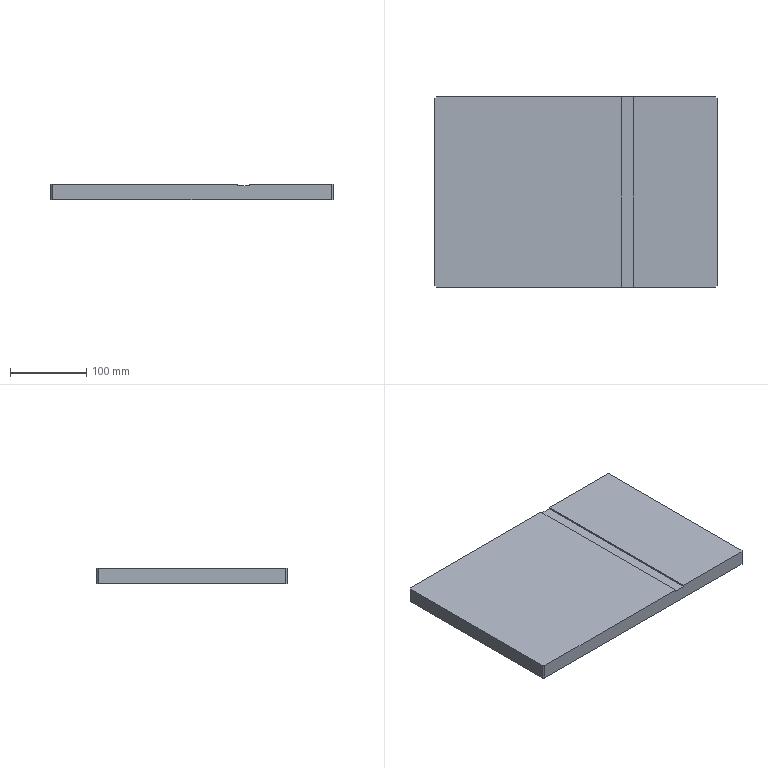Part | STEP file | 001-003-Storage mechanism base plate | 1 solid | 14 faces | box 370 x 250 x 20 mm | volume 1842340 mm3 | plane 14
STEP:
#1=CARTESIAN_POINT('',(0.,0.,0.));
#2=DIRECTION('',(0.,0.,1.));
#3=DIRECTION('',(1.,0.,0.));
#4=AXIS2_PLACEMENT_3D('',#1,#2,#3);
#5=CARTESIAN_POINT('',(183.,125.,20.));
#6=VERTEX_POINT('',#5);
#7=CARTESIAN_POINT('',(75.,125.,20.));
#8=VERTEX_POINT('',#7);
#9=CARTESIAN_POINT('',(-185.,125.,20.));
#10=DIRECTION('',(-1.,0.,0.));
#11=VECTOR('',#10,1.);
#12=LINE('',#9,#11);
#13=CARTESIAN_POINT('',(0.,0.,20.));
#14=DIRECTION('',(0.,0.,-1.));
#15=DIRECTION('',(-1.,0.,0.));
#16=AXIS2_PLACEMENT_3D('',#13,#14,#15);
#17=PLANE('',#16);
#18=CARTESIAN_POINT('',(185.,125.));
#19=DIRECTION('',(1.,0.));
#20=VECTOR('',#19,1.);
#21=LINE('',#18,#20);
#22=(GEOMETRIC_REPRESENTATION_CONTEXT(2)PARAMETRIC_REPRESENTATION_CONTEXT()REPRESENTATION_CONTEXT('',''));
#23=DEFINITIONAL_REPRESENTATION('',(#21),#22);
#24=PCURVE('',#17,#23);
#25=CARTESIAN_POINT('',(-185.,125.,20.));
#26=DIRECTION('',(0.,-1.,0.));
#27=DIRECTION('',(0.,0.,-1.));
#28=AXIS2_PLACEMENT_3D('',#25,#26,#27);
#29=PLANE('',#28);
#30=CARTESIAN_POINT('',(0.,0.));
#31=DIRECTION('',(0.,-1.));
#32=VECTOR('',#31,1.);
#33=LINE('',#30,#32);
#34=(GEOMETRIC_REPRESENTATION_CONTEXT(2)PARAMETRIC_REPRESENTATION_CONTEXT()REPRESENTATION_CONTEXT('',''));
#35=DEFINITIONAL_REPRESENTATION('',(#33),#34);
#36=PCURVE('',#29,#35);
#37=SURFACE_CURVE('',#12,(#24,#36),.PCURVE_S1.);
#38=EDGE_CURVE('',#6,#8,#37,.T.);
#39=ORIENTED_EDGE('',*,*,#38,.T.);
#40=CARTESIAN_POINT('',(75.,-125.,20.));
#41=VERTEX_POINT('',#40);
#42=CARTESIAN_POINT('',(75.,125.,20.));
#43=DIRECTION('',(0.,1.,0.));
#44=VECTOR('',#43,1.);
#45=LINE('',#42,#44);
#46=CARTESIAN_POINT('',(-75.,125.));
#47=DIRECTION('',(0.,1.));
#48=VECTOR('',#47,1.);
#49=LINE('',#46,#48);
#50=(GEOMETRIC_REPRESENTATION_CONTEXT(2)PARAMETRIC_REPRESENTATION_CONTEXT()REPRESENTATION_CONTEXT('',''));
#51=DEFINITIONAL_REPRESENTATION('',(#49),#50);
#52=PCURVE('',#17,#51);
#53=CARTESIAN_POINT('',(75.,125.,18.));
#54=DIRECTION('',(1.,0.,0.));
#55=DIRECTION('',(0.,1.,0.));
#56=AXIS2_PLACEMENT_3D('',#53,#54,#55);
#57=PLANE('',#56);
#58=CARTESIAN_POINT('',(0.,2.));
#59=DIRECTION('',(1.,0.));
#60=VECTOR('',#59,1.);
#61=LINE('',#58,#60);
#62=(GEOMETRIC_REPRESENTATION_CONTEXT(2)PARAMETRIC_REPRESENTATION_CONTEXT()REPRESENTATION_CONTEXT('',''));
#63=DEFINITIONAL_REPRESENTATION('',(#61),#62);
#64=PCURVE('',#57,#63);
#65=SURFACE_CURVE('',#45,(#52,#64),.PCURVE_S1.);
#66=EDGE_CURVE('',#41,#8,#65,.T.);
#67=ORIENTED_EDGE('',*,*,#66,.F.);
#68=CARTESIAN_POINT('',(183.,-125.,20.));
#69=VERTEX_POINT('',#68);
#70=CARTESIAN_POINT('',(-185.,-125.,20.));
#71=DIRECTION('',(1.,0.,0.));
#72=VECTOR('',#71,1.);
#73=LINE('',#70,#72);
#74=CARTESIAN_POINT('',(185.,-125.));
#75=DIRECTION('',(-1.,0.));
#76=VECTOR('',#75,1.);
#77=LINE('',#74,#76);
#78=(GEOMETRIC_REPRESENTATION_CONTEXT(2)PARAMETRIC_REPRESENTATION_CONTEXT()REPRESENTATION_CONTEXT('',''));
#79=DEFINITIONAL_REPRESENTATION('',(#77),#78);
#80=PCURVE('',#17,#79);
#81=CARTESIAN_POINT('',(-185.,-125.,20.));
#82=DIRECTION('',(0.,1.,0.));
#83=DIRECTION('',(0.,0.,1.));
#84=AXIS2_PLACEMENT_3D('',#81,#82,#83);
#85=PLANE('',#84);
#86=CARTESIAN_POINT('',(0.,0.));
#87=DIRECTION('',(0.,1.));
#88=VECTOR('',#87,1.);
#89=LINE('',#86,#88);
#90=(GEOMETRIC_REPRESENTATION_CONTEXT(2)PARAMETRIC_REPRESENTATION_CONTEXT()REPRESENTATION_CONTEXT('',''));
#91=DEFINITIONAL_REPRESENTATION('',(#89),#90);
#92=PCURVE('',#85,#91);
#93=SURFACE_CURVE('',#73,(#80,#92),.PCURVE_S1.);
#94=EDGE_CURVE('',#41,#69,#93,.T.);
#95=ORIENTED_EDGE('',*,*,#94,.T.);
#96=CARTESIAN_POINT('',(185.,-123.,20.));
#97=VERTEX_POINT('',#96);
#98=CARTESIAN_POINT('',(185.,-123.,20.));
#99=DIRECTION('',(0.7071,0.7071,0.));
#100=VECTOR('',#99,1.);
#101=LINE('',#98,#100);
#102=CARTESIAN_POINT('',(-185.,-123.));
#103=DIRECTION('',(-0.7071,0.7071));
#104=VECTOR('',#103,1.);
#105=LINE('',#102,#104);
#106=(GEOMETRIC_REPRESENTATION_CONTEXT(2)PARAMETRIC_REPRESENTATION_CONTEXT()REPRESENTATION_CONTEXT('',''));
#107=DEFINITIONAL_REPRESENTATION('',(#105),#106);
#108=PCURVE('',#17,#107);
#109=CARTESIAN_POINT('',(185.,-123.,20.));
#110=DIRECTION('',(-0.7071,0.7071,0.));
#111=DIRECTION('',(0.,0.,-1.));
#112=AXIS2_PLACEMENT_3D('',#109,#110,#111);
#113=PLANE('',#112);
#114=CARTESIAN_POINT('',(0.,0.));
#115=DIRECTION('',(0.,-1.));
#116=VECTOR('',#115,1.);
#117=LINE('',#114,#116);
#118=(GEOMETRIC_REPRESENTATION_CONTEXT(2)PARAMETRIC_REPRESENTATION_CONTEXT()REPRESENTATION_CONTEXT('',''));
#119=DEFINITIONAL_REPRESENTATION('',(#117),#118);
#120=PCURVE('',#113,#119);
#121=SURFACE_CURVE('',#101,(#108,#120),.PCURVE_S1.);
#122=EDGE_CURVE('',#69,#97,#121,.T.);
#123=ORIENTED_EDGE('',*,*,#122,.T.);
#124=CARTESIAN_POINT('',(185.,123.,20.));
#125=VERTEX_POINT('',#124);
#126=CARTESIAN_POINT('',(185.,-125.,20.));
#127=DIRECTION('',(0.,1.,0.));
#128=VECTOR('',#127,1.);
#129=LINE('',#126,#128);
#130=CARTESIAN_POINT('',(-185.,-125.));
#131=DIRECTION('',(0.,1.));
#132=VECTOR('',#131,1.);
#133=LINE('',#130,#132);
#134=(GEOMETRIC_REPRESENTATION_CONTEXT(2)PARAMETRIC_REPRESENTATION_CONTEXT()REPRESENTATION_CONTEXT('',''));
#135=DEFINITIONAL_REPRESENTATION('',(#133),#134);
#136=PCURVE('',#17,#135);
#137=CARTESIAN_POINT('',(185.,-125.,20.));
#138=DIRECTION('',(-1.,0.,0.));
#139=DIRECTION('',(0.,0.,1.));
#140=AXIS2_PLACEMENT_3D('',#137,#138,#139);
#141=PLANE('',#140);
#142=CARTESIAN_POINT('',(0.,0.));
#143=DIRECTION('',(0.,1.));
#144=VECTOR('',#143,1.);
#145=LINE('',#142,#144);
#146=(GEOMETRIC_REPRESENTATION_CONTEXT(2)PARAMETRIC_REPRESENTATION_CONTEXT()REPRESENTATION_CONTEXT('',''));
#147=DEFINITIONAL_REPRESENTATION('',(#145),#146);
#148=PCURVE('',#141,#147);
#149=SURFACE_CURVE('',#129,(#136,#148),.PCURVE_S1.);
#150=EDGE_CURVE('',#97,#125,#149,.T.);
#151=ORIENTED_EDGE('',*,*,#150,.T.);
#152=CARTESIAN_POINT('',(183.,125.,20.));
#153=DIRECTION('',(-0.7071,0.7071,0.));
#154=VECTOR('',#153,1.);
#155=LINE('',#152,#154);
#156=CARTESIAN_POINT('',(-183.,125.));
#157=DIRECTION('',(0.7071,0.7071));
#158=VECTOR('',#157,1.);
#159=LINE('',#156,#158);
#160=(GEOMETRIC_REPRESENTATION_CONTEXT(2)PARAMETRIC_REPRESENTATION_CONTEXT()REPRESENTATION_CONTEXT('',''));
#161=DEFINITIONAL_REPRESENTATION('',(#159),#160);
#162=PCURVE('',#17,#161);
#163=CARTESIAN_POINT('',(183.,125.,20.));
#164=DIRECTION('',(-0.7071,-0.7071,0.));
#165=DIRECTION('',(0.,0.,-1.));
#166=AXIS2_PLACEMENT_3D('',#163,#164,#165);
#167=PLANE('',#166);
#168=CARTESIAN_POINT('',(0.,0.));
#169=DIRECTION('',(0.,-1.));
#170=VECTOR('',#169,1.);
#171=LINE('',#168,#170);
#172=(GEOMETRIC_REPRESENTATION_CONTEXT(2)PARAMETRIC_REPRESENTATION_CONTEXT()REPRESENTATION_CONTEXT('',''));
#173=DEFINITIONAL_REPRESENTATION('',(#171),#172);
#174=PCURVE('',#167,#173);
#175=SURFACE_CURVE('',#155,(#162,#174),.PCURVE_S1.);
#176=EDGE_CURVE('',#125,#6,#175,.T.);
#177=ORIENTED_EDGE('',*,*,#176,.T.);
#178=EDGE_LOOP('',(#39,#67,#95,#123,#151,#177));
#179=FACE_BOUND('',#178,.T.);
#180=ADVANCED_FACE('',(#179),#17,.F.);
#181=ORIENTED_EDGE('',*,*,#150,.F.);
#182=CARTESIAN_POINT('',(185.,-123.,0.));
#183=VERTEX_POINT('',#182);
#184=CARTESIAN_POINT('',(185.,-123.,20.));
#185=DIRECTION('',(0.,0.,-1.));
#186=VECTOR('',#185,1.);
#187=LINE('',#184,#186);
#188=CARTESIAN_POINT('',(0.,2.));
#189=DIRECTION('',(-1.,0.));
#190=VECTOR('',#189,1.);
#191=LINE('',#188,#190);
#192=(GEOMETRIC_REPRESENTATION_CONTEXT(2)PARAMETRIC_REPRESENTATION_CONTEXT()REPRESENTATION_CONTEXT('',''));
#193=DEFINITIONAL_REPRESENTATION('',(#191),#192);
#194=PCURVE('',#141,#193);
#195=CARTESIAN_POINT('',(0.,0.));
#196=DIRECTION('',(1.,0.));
#197=VECTOR('',#196,1.);
#198=LINE('',#195,#197);
#199=(GEOMETRIC_REPRESENTATION_CONTEXT(2)PARAMETRIC_REPRESENTATION_CONTEXT()REPRESENTATION_CONTEXT('',''));
#200=DEFINITIONAL_REPRESENTATION('',(#198),#199);
#201=PCURVE('',#113,#200);
#202=SURFACE_CURVE('',#187,(#194,#201),.PCURVE_S1.);
#203=EDGE_CURVE('',#97,#183,#202,.T.);
#204=ORIENTED_EDGE('',*,*,#203,.T.);
#205=CARTESIAN_POINT('',(185.,123.,0.));
#206=VERTEX_POINT('',#205);
#207=CARTESIAN_POINT('',(185.,-125.,0.));
#208=DIRECTION('',(0.,1.,0.));
#209=VECTOR('',#208,1.);
#210=LINE('',#207,#209);
#211=CARTESIAN_POINT('',(-20.,0.));
#212=DIRECTION('',(0.,1.));
#213=VECTOR('',#212,1.);
#214=LINE('',#211,#213);
#215=(GEOMETRIC_REPRESENTATION_CONTEXT(2)PARAMETRIC_REPRESENTATION_CONTEXT()REPRESENTATION_CONTEXT('',''));
#216=DEFINITIONAL_REPRESENTATION('',(#214),#215);
#217=PCURVE('',#141,#216);
#218=CARTESIAN_POINT('',(0.,0.,0.));
#219=DIRECTION('',(0.,0.,-1.));
#220=DIRECTION('',(-1.,0.,0.));
#221=AXIS2_PLACEMENT_3D('',#218,#219,#220);
#222=PLANE('',#221);
#223=CARTESIAN_POINT('',(-185.,-125.));
#224=DIRECTION('',(0.,1.));
#225=VECTOR('',#224,1.);
#226=LINE('',#223,#225);
#227=(GEOMETRIC_REPRESENTATION_CONTEXT(2)PARAMETRIC_REPRESENTATION_CONTEXT()REPRESENTATION_CONTEXT('',''));
#228=DEFINITIONAL_REPRESENTATION('',(#226),#227);
#229=PCURVE('',#222,#228);
#230=SURFACE_CURVE('',#210,(#217,#229),.PCURVE_S1.);
#231=EDGE_CURVE('',#183,#206,#230,.T.);
#232=ORIENTED_EDGE('',*,*,#231,.T.);
#233=CARTESIAN_POINT('',(185.,123.,20.));
#234=DIRECTION('',(0.,0.,1.));
#235=VECTOR('',#234,1.);
#236=LINE('',#233,#235);
#237=CARTESIAN_POINT('',(0.,248.));
#238=DIRECTION('',(1.,0.));
#239=VECTOR('',#238,1.);
#240=LINE('',#237,#239);
#241=(GEOMETRIC_REPRESENTATION_CONTEXT(2)PARAMETRIC_REPRESENTATION_CONTEXT()REPRESENTATION_CONTEXT('',''));
#242=DEFINITIONAL_REPRESENTATION('',(#240),#241);
#243=PCURVE('',#141,#242);
#244=CARTESIAN_POINT('',(0.,2.828));
#245=DIRECTION('',(-1.,0.));
#246=VECTOR('',#245,1.);
#247=LINE('',#244,#246);
#248=(GEOMETRIC_REPRESENTATION_CONTEXT(2)PARAMETRIC_REPRESENTATION_CONTEXT()REPRESENTATION_CONTEXT('',''));
#249=DEFINITIONAL_REPRESENTATION('',(#247),#248);
#250=PCURVE('',#167,#249);
#251=SURFACE_CURVE('',#236,(#243,#250),.PCURVE_S1.);
#252=EDGE_CURVE('',#206,#125,#251,.T.);
#253=ORIENTED_EDGE('',*,*,#252,.T.);
#254=EDGE_LOOP('',(#181,#204,#232,#253));
#255=FACE_BOUND('',#254,.T.);
#256=ADVANCED_FACE('',(#255),#141,.F.);
#257=CARTESIAN_POINT('',(75.,125.,18.));
#258=VERTEX_POINT('',#257);
#259=CARTESIAN_POINT('',(60.,125.,18.));
#260=VERTEX_POINT('',#259);
#261=CARTESIAN_POINT('',(75.,125.,18.));
#262=DIRECTION('',(-1.,0.,0.));
#263=VECTOR('',#262,1.);
#264=LINE('',#261,#263);
#265=CARTESIAN_POINT('',(2.,260.));
#266=DIRECTION('',(0.,-1.));
#267=VECTOR('',#266,1.);
#268=LINE('',#265,#267);
#269=(GEOMETRIC_REPRESENTATION_CONTEXT(2)PARAMETRIC_REPRESENTATION_CONTEXT()REPRESENTATION_CONTEXT('',''));
#270=DEFINITIONAL_REPRESENTATION('',(#268),#269);
#271=PCURVE('',#29,#270);
#272=CARTESIAN_POINT('',(0.,0.,18.));
#273=DIRECTION('',(0.,0.,-1.));
#274=DIRECTION('',(-1.,0.,0.));
#275=AXIS2_PLACEMENT_3D('',#272,#273,#274);
#276=PLANE('',#275);
#277=CARTESIAN_POINT('',(-75.,125.));
#278=DIRECTION('',(1.,0.));
#279=VECTOR('',#278,1.);
#280=LINE('',#277,#279);
#281=(GEOMETRIC_REPRESENTATION_CONTEXT(2)PARAMETRIC_REPRESENTATION_CONTEXT()REPRESENTATION_CONTEXT('',''));
#282=DEFINITIONAL_REPRESENTATION('',(#280),#281);
#283=PCURVE('',#276,#282);
#284=SURFACE_CURVE('',#264,(#271,#283),.PCURVE_S1.);
#285=EDGE_CURVE('',#258,#260,#284,.T.);
#286=ORIENTED_EDGE('',*,*,#285,.F.);
#287=CARTESIAN_POINT('',(75.,125.,18.));
#288=DIRECTION('',(0.,0.,1.));
#289=VECTOR('',#288,1.);
#290=LINE('',#287,#289);
#291=CARTESIAN_POINT('',(2.,260.));
#292=DIRECTION('',(-1.,0.));
#293=VECTOR('',#292,1.);
#294=LINE('',#291,#293);
#295=(GEOMETRIC_REPRESENTATION_CONTEXT(2)PARAMETRIC_REPRESENTATION_CONTEXT()REPRESENTATION_CONTEXT('',''));
#296=DEFINITIONAL_REPRESENTATION('',(#294),#295);
#297=PCURVE('',#29,#296);
#298=CARTESIAN_POINT('',(0.,0.));
#299=DIRECTION('',(0.,1.));
#300=VECTOR('',#299,1.);
#301=LINE('',#298,#300);
#302=(GEOMETRIC_REPRESENTATION_CONTEXT(2)PARAMETRIC_REPRESENTATION_CONTEXT()REPRESENTATION_CONTEXT('',''));
#303=DEFINITIONAL_REPRESENTATION('',(#301),#302);
#304=PCURVE('',#57,#303);
#305=SURFACE_CURVE('',#290,(#297,#304),.PCURVE_S1.);
#306=EDGE_CURVE('',#258,#8,#305,.T.);
#307=ORIENTED_EDGE('',*,*,#306,.T.);
#308=ORIENTED_EDGE('',*,*,#38,.F.);
#309=CARTESIAN_POINT('',(183.,125.,0.));
#310=VERTEX_POINT('',#309);
#311=CARTESIAN_POINT('',(183.,125.,20.));
#312=DIRECTION('',(0.,0.,-1.));
#313=VECTOR('',#312,1.);
#314=LINE('',#311,#313);
#315=CARTESIAN_POINT('',(0.,368.));
#316=DIRECTION('',(1.,0.));
#317=VECTOR('',#316,1.);
#318=LINE('',#315,#317);
#319=(GEOMETRIC_REPRESENTATION_CONTEXT(2)PARAMETRIC_REPRESENTATION_CONTEXT()REPRESENTATION_CONTEXT('',''));
#320=DEFINITIONAL_REPRESENTATION('',(#318),#319);
#321=PCURVE('',#29,#320);
#322=CARTESIAN_POINT('',(0.,0.));
#323=DIRECTION('',(1.,0.));
#324=VECTOR('',#323,1.);
#325=LINE('',#322,#324);
#326=(GEOMETRIC_REPRESENTATION_CONTEXT(2)PARAMETRIC_REPRESENTATION_CONTEXT()REPRESENTATION_CONTEXT('',''));
#327=DEFINITIONAL_REPRESENTATION('',(#325),#326);
#328=PCURVE('',#167,#327);
#329=SURFACE_CURVE('',#314,(#321,#328),.PCURVE_S1.);
#330=EDGE_CURVE('',#6,#310,#329,.T.);
#331=ORIENTED_EDGE('',*,*,#330,.T.);
#332=CARTESIAN_POINT('',(-183.,125.,0.));
#333=VERTEX_POINT('',#332);
#334=CARTESIAN_POINT('',(-185.,125.,0.));
#335=DIRECTION('',(-1.,0.,0.));
#336=VECTOR('',#335,1.);
#337=LINE('',#334,#336);
#338=CARTESIAN_POINT('',(20.,0.));
#339=DIRECTION('',(0.,-1.));
#340=VECTOR('',#339,1.);
#341=LINE('',#338,#340);
#342=(GEOMETRIC_REPRESENTATION_CONTEXT(2)PARAMETRIC_REPRESENTATION_CONTEXT()REPRESENTATION_CONTEXT('',''));
#343=DEFINITIONAL_REPRESENTATION('',(#341),#342);
#344=PCURVE('',#29,#343);
#345=CARTESIAN_POINT('',(185.,125.));
#346=DIRECTION('',(1.,0.));
#347=VECTOR('',#346,1.);
#348=LINE('',#345,#347);
#349=(GEOMETRIC_REPRESENTATION_CONTEXT(2)PARAMETRIC_REPRESENTATION_CONTEXT()REPRESENTATION_CONTEXT('',''));
#350=DEFINITIONAL_REPRESENTATION('',(#348),#349);
#351=PCURVE('',#222,#350);
#352=SURFACE_CURVE('',#337,(#344,#351),.PCURVE_S1.);
#353=EDGE_CURVE('',#310,#333,#352,.T.);
#354=ORIENTED_EDGE('',*,*,#353,.T.);
#355=CARTESIAN_POINT('',(-183.,125.,20.));
#356=VERTEX_POINT('',#355);
#357=CARTESIAN_POINT('',(-183.,125.,20.));
#358=DIRECTION('',(0.,0.,1.));
#359=VECTOR('',#358,1.);
#360=LINE('',#357,#359);
#361=CARTESIAN_POINT('',(0.,2.));
#362=DIRECTION('',(-1.,0.));
#363=VECTOR('',#362,1.);
#364=LINE('',#361,#363);
#365=(GEOMETRIC_REPRESENTATION_CONTEXT(2)PARAMETRIC_REPRESENTATION_CONTEXT()REPRESENTATION_CONTEXT('',''));
#366=DEFINITIONAL_REPRESENTATION('',(#364),#365);
#367=PCURVE('',#29,#366);
#368=CARTESIAN_POINT('',(-185.,123.,20.));
#369=DIRECTION('',(0.7071,-0.7071,0.));
#370=DIRECTION('',(0.,0.,-1.));
#371=AXIS2_PLACEMENT_3D('',#368,#369,#370);
#372=PLANE('',#371);
#373=CARTESIAN_POINT('',(0.,2.828));
#374=DIRECTION('',(-1.,0.));
#375=VECTOR('',#374,1.);
#376=LINE('',#373,#375);
#377=(GEOMETRIC_REPRESENTATION_CONTEXT(2)PARAMETRIC_REPRESENTATION_CONTEXT()REPRESENTATION_CONTEXT('',''));
#378=DEFINITIONAL_REPRESENTATION('',(#376),#377);
#379=PCURVE('',#372,#378);
#380=SURFACE_CURVE('',#360,(#367,#379),.PCURVE_S1.);
#381=EDGE_CURVE('',#333,#356,#380,.T.);
#382=ORIENTED_EDGE('',*,*,#381,.T.);
#383=CARTESIAN_POINT('',(60.,125.,20.));
#384=VERTEX_POINT('',#383);
#385=CARTESIAN_POINT('',(-185.,125.,20.));
#386=DIRECTION('',(-1.,0.,0.));
#387=VECTOR('',#386,1.);
#388=LINE('',#385,#387);
#389=CARTESIAN_POINT('',(0.,0.));
#390=DIRECTION('',(0.,-1.));
#391=VECTOR('',#390,1.);
#392=LINE('',#389,#391);
#393=(GEOMETRIC_REPRESENTATION_CONTEXT(2)PARAMETRIC_REPRESENTATION_CONTEXT()REPRESENTATION_CONTEXT('',''));
#394=DEFINITIONAL_REPRESENTATION('',(#392),#393);
#395=PCURVE('',#29,#394);
#396=CARTESIAN_POINT('',(0.,0.,20.));
#397=DIRECTION('',(0.,0.,-1.));
#398=DIRECTION('',(-1.,0.,0.));
#399=AXIS2_PLACEMENT_3D('',#396,#397,#398);
#400=PLANE('',#399);
#401=CARTESIAN_POINT('',(185.,125.));
#402=DIRECTION('',(1.,0.));
#403=VECTOR('',#402,1.);
#404=LINE('',#401,#403);
#405=(GEOMETRIC_REPRESENTATION_CONTEXT(2)PARAMETRIC_REPRESENTATION_CONTEXT()REPRESENTATION_CONTEXT('',''));
#406=DEFINITIONAL_REPRESENTATION('',(#404),#405);
#407=PCURVE('',#400,#406);
#408=SURFACE_CURVE('',#388,(#395,#407),.PCURVE_S1.);
#409=EDGE_CURVE('',#384,#356,#408,.T.);
#410=ORIENTED_EDGE('',*,*,#409,.F.);
#411=CARTESIAN_POINT('',(60.,125.,18.));
#412=DIRECTION('',(0.,0.,1.));
#413=VECTOR('',#412,1.);
#414=LINE('',#411,#413);
#415=CARTESIAN_POINT('',(2.,245.));
#416=DIRECTION('',(-1.,0.));
#417=VECTOR('',#416,1.);
#418=LINE('',#415,#417);
#419=(GEOMETRIC_REPRESENTATION_CONTEXT(2)PARAMETRIC_REPRESENTATION_CONTEXT()REPRESENTATION_CONTEXT('',''));
#420=DEFINITIONAL_REPRESENTATION('',(#418),#419);
#421=PCURVE('',#29,#420);
#422=CARTESIAN_POINT('',(60.,125.,18.));
#423=DIRECTION('',(-1.,0.,0.));
#424=DIRECTION('',(0.,-1.,0.));
#425=AXIS2_PLACEMENT_3D('',#422,#423,#424);
#426=PLANE('',#425);
#427=CARTESIAN_POINT('',(0.,0.));
#428=DIRECTION('',(0.,1.));
#429=VECTOR('',#428,1.);
#430=LINE('',#427,#429);
#431=(GEOMETRIC_REPRESENTATION_CONTEXT(2)PARAMETRIC_REPRESENTATION_CONTEXT()REPRESENTATION_CONTEXT('',''));
#432=DEFINITIONAL_REPRESENTATION('',(#430),#431);
#433=PCURVE('',#426,#432);
#434=SURFACE_CURVE('',#414,(#421,#433),.PCURVE_S1.);
#435=EDGE_CURVE('',#260,#384,#434,.T.);
#436=ORIENTED_EDGE('',*,*,#435,.F.);
#437=EDGE_LOOP('',(#286,#307,#308,#331,#354,#382,#410,#436));
#438=FACE_BOUND('',#437,.T.);
#439=ADVANCED_FACE('',(#438),#29,.F.);
#440=CARTESIAN_POINT('',(-185.,123.,0.));
#441=VERTEX_POINT('',#440);
#442=CARTESIAN_POINT('',(-185.,-123.,0.));
#443=VERTEX_POINT('',#442);
#444=CARTESIAN_POINT('',(-185.,-125.,0.));
#445=DIRECTION('',(0.,-1.,0.));
#446=VECTOR('',#445,1.);
#447=LINE('',#444,#446);
#448=CARTESIAN_POINT('',(-185.,-125.,20.));
#449=DIRECTION('',(1.,0.,0.));
#450=DIRECTION('',(0.,0.,-1.));
#451=AXIS2_PLACEMENT_3D('',#448,#449,#450);
#452=PLANE('',#451);
#453=CARTESIAN_POINT('',(20.,0.));
#454=DIRECTION('',(0.,-1.));
#455=VECTOR('',#454,1.);
#456=LINE('',#453,#455);
#457=(GEOMETRIC_REPRESENTATION_CONTEXT(2)PARAMETRIC_REPRESENTATION_CONTEXT()REPRESENTATION_CONTEXT('',''));
#458=DEFINITIONAL_REPRESENTATION('',(#456),#457);
#459=PCURVE('',#452,#458);
#460=CARTESIAN_POINT('',(185.,-125.));
#461=DIRECTION('',(0.,-1.));
#462=VECTOR('',#461,1.);
#463=LINE('',#460,#462);
#464=(GEOMETRIC_REPRESENTATION_CONTEXT(2)PARAMETRIC_REPRESENTATION_CONTEXT()REPRESENTATION_CONTEXT('',''));
#465=DEFINITIONAL_REPRESENTATION('',(#463),#464);
#466=PCURVE('',#222,#465);
#467=SURFACE_CURVE('',#447,(#459,#466),.PCURVE_S1.);
#468=EDGE_CURVE('',#441,#443,#467,.T.);
#469=ORIENTED_EDGE('',*,*,#468,.T.);
#470=CARTESIAN_POINT('',(-185.,-123.,20.));
#471=VERTEX_POINT('',#470);
#472=CARTESIAN_POINT('',(-185.,-123.,20.));
#473=DIRECTION('',(0.,0.,1.));
#474=VECTOR('',#473,1.);
#475=LINE('',#472,#474);
#476=CARTESIAN_POINT('',(0.,2.));
#477=DIRECTION('',(-1.,0.));
#478=VECTOR('',#477,1.);
#479=LINE('',#476,#478);
#480=(GEOMETRIC_REPRESENTATION_CONTEXT(2)PARAMETRIC_REPRESENTATION_CONTEXT()REPRESENTATION_CONTEXT('',''));
#481=DEFINITIONAL_REPRESENTATION('',(#479),#480);
#482=PCURVE('',#452,#481);
#483=CARTESIAN_POINT('',(-183.,-125.,20.));
#484=DIRECTION('',(0.7071,0.7071,0.));
#485=DIRECTION('',(0.,0.,-1.));
#486=AXIS2_PLACEMENT_3D('',#483,#484,#485);
#487=PLANE('',#486);
#488=CARTESIAN_POINT('',(0.,2.828));
#489=DIRECTION('',(-1.,0.));
#490=VECTOR('',#489,1.);
#491=LINE('',#488,#490);
#492=(GEOMETRIC_REPRESENTATION_CONTEXT(2)PARAMETRIC_REPRESENTATION_CONTEXT()REPRESENTATION_CONTEXT('',''));
#493=DEFINITIONAL_REPRESENTATION('',(#491),#492);
#494=PCURVE('',#487,#493);
#495=SURFACE_CURVE('',#475,(#482,#494),.PCURVE_S1.);
#496=EDGE_CURVE('',#443,#471,#495,.T.);
#497=ORIENTED_EDGE('',*,*,#496,.T.);
#498=CARTESIAN_POINT('',(-185.,123.,20.));
#499=VERTEX_POINT('',#498);
#500=CARTESIAN_POINT('',(-185.,-125.,20.));
#501=DIRECTION('',(0.,-1.,0.));
#502=VECTOR('',#501,1.);
#503=LINE('',#500,#502);
#504=CARTESIAN_POINT('',(0.,0.));
#505=DIRECTION('',(0.,-1.));
#506=VECTOR('',#505,1.);
#507=LINE('',#504,#506);
#508=(GEOMETRIC_REPRESENTATION_CONTEXT(2)PARAMETRIC_REPRESENTATION_CONTEXT()REPRESENTATION_CONTEXT('',''));
#509=DEFINITIONAL_REPRESENTATION('',(#507),#508);
#510=PCURVE('',#452,#509);
#511=CARTESIAN_POINT('',(185.,-125.));
#512=DIRECTION('',(0.,-1.));
#513=VECTOR('',#512,1.);
#514=LINE('',#511,#513);
#515=(GEOMETRIC_REPRESENTATION_CONTEXT(2)PARAMETRIC_REPRESENTATION_CONTEXT()REPRESENTATION_CONTEXT('',''));
#516=DEFINITIONAL_REPRESENTATION('',(#514),#515);
#517=PCURVE('',#400,#516);
#518=SURFACE_CURVE('',#503,(#510,#517),.PCURVE_S1.);
#519=EDGE_CURVE('',#499,#471,#518,.T.);
#520=ORIENTED_EDGE('',*,*,#519,.F.);
#521=CARTESIAN_POINT('',(-185.,123.,20.));
#522=DIRECTION('',(0.,0.,-1.));
#523=VECTOR('',#522,1.);
#524=LINE('',#521,#523);
#525=CARTESIAN_POINT('',(0.,248.));
#526=DIRECTION('',(1.,0.));
#527=VECTOR('',#526,1.);
#528=LINE('',#525,#527);
#529=(GEOMETRIC_REPRESENTATION_CONTEXT(2)PARAMETRIC_REPRESENTATION_CONTEXT()REPRESENTATION_CONTEXT('',''));
#530=DEFINITIONAL_REPRESENTATION('',(#528),#529);
#531=PCURVE('',#452,#530);
#532=CARTESIAN_POINT('',(0.,0.));
#533=DIRECTION('',(1.,0.));
#534=VECTOR('',#533,1.);
#535=LINE('',#532,#534);
#536=(GEOMETRIC_REPRESENTATION_CONTEXT(2)PARAMETRIC_REPRESENTATION_CONTEXT()REPRESENTATION_CONTEXT('',''));
#537=DEFINITIONAL_REPRESENTATION('',(#535),#536);
#538=PCURVE('',#372,#537);
#539=SURFACE_CURVE('',#524,(#531,#538),.PCURVE_S1.);
#540=EDGE_CURVE('',#499,#441,#539,.T.);
#541=ORIENTED_EDGE('',*,*,#540,.T.);
#542=EDGE_LOOP('',(#469,#497,#520,#541));
#543=FACE_BOUND('',#542,.T.);
#544=ADVANCED_FACE('',(#543),#452,.F.);
#545=ORIENTED_EDGE('',*,*,#94,.F.);
#546=CARTESIAN_POINT('',(75.,-125.,18.));
#547=VERTEX_POINT('',#546);
#548=CARTESIAN_POINT('',(75.,-125.,18.));
#549=DIRECTION('',(0.,0.,1.));
#550=VECTOR('',#549,1.);
#551=LINE('',#548,#550);
#552=CARTESIAN_POINT('',(-2.,260.));
#553=DIRECTION('',(1.,0.));
#554=VECTOR('',#553,1.);
#555=LINE('',#552,#554);
#556=(GEOMETRIC_REPRESENTATION_CONTEXT(2)PARAMETRIC_REPRESENTATION_CONTEXT()REPRESENTATION_CONTEXT('',''));
#557=DEFINITIONAL_REPRESENTATION('',(#555),#556);
#558=PCURVE('',#85,#557);
#559=CARTESIAN_POINT('',(-250.,0.));
#560=DIRECTION('',(0.,1.));
#561=VECTOR('',#560,1.);
#562=LINE('',#559,#561);
#563=(GEOMETRIC_REPRESENTATION_CONTEXT(2)PARAMETRIC_REPRESENTATION_CONTEXT()REPRESENTATION_CONTEXT('',''));
#564=DEFINITIONAL_REPRESENTATION('',(#562),#563);
#565=PCURVE('',#57,#564);
#566=SURFACE_CURVE('',#551,(#558,#565),.PCURVE_S1.);
#567=EDGE_CURVE('',#547,#41,#566,.T.);
#568=ORIENTED_EDGE('',*,*,#567,.F.);
#569=CARTESIAN_POINT('',(60.,-125.,18.));
#570=VERTEX_POINT('',#569);
#571=CARTESIAN_POINT('',(75.,-125.,18.));
#572=DIRECTION('',(1.,0.,0.));
#573=VECTOR('',#572,1.);
#574=LINE('',#571,#573);
#575=CARTESIAN_POINT('',(-2.,260.));
#576=DIRECTION('',(0.,1.));
#577=VECTOR('',#576,1.);
#578=LINE('',#575,#577);
#579=(GEOMETRIC_REPRESENTATION_CONTEXT(2)PARAMETRIC_REPRESENTATION_CONTEXT()REPRESENTATION_CONTEXT('',''));
#580=DEFINITIONAL_REPRESENTATION('',(#578),#579);
#581=PCURVE('',#85,#580);
#582=CARTESIAN_POINT('',(-75.,-125.));
#583=DIRECTION('',(-1.,0.));
#584=VECTOR('',#583,1.);
#585=LINE('',#582,#584);
#586=(GEOMETRIC_REPRESENTATION_CONTEXT(2)PARAMETRIC_REPRESENTATION_CONTEXT()REPRESENTATION_CONTEXT('',''));
#587=DEFINITIONAL_REPRESENTATION('',(#585),#586);
#588=PCURVE('',#276,#587);
#589=SURFACE_CURVE('',#574,(#581,#588),.PCURVE_S1.);
#590=EDGE_CURVE('',#570,#547,#589,.T.);
#591=ORIENTED_EDGE('',*,*,#590,.F.);
#592=CARTESIAN_POINT('',(60.,-125.,20.));
#593=VERTEX_POINT('',#592);
#594=CARTESIAN_POINT('',(60.,-125.,18.));
#595=DIRECTION('',(0.,0.,1.));
#596=VECTOR('',#595,1.);
#597=LINE('',#594,#596);
#598=CARTESIAN_POINT('',(-2.,245.));
#599=DIRECTION('',(1.,0.));
#600=VECTOR('',#599,1.);
#601=LINE('',#598,#600);
#602=(GEOMETRIC_REPRESENTATION_CONTEXT(2)PARAMETRIC_REPRESENTATION_CONTEXT()REPRESENTATION_CONTEXT('',''));
#603=DEFINITIONAL_REPRESENTATION('',(#601),#602);
#604=PCURVE('',#85,#603);
#605=CARTESIAN_POINT('',(250.,0.));
#606=DIRECTION('',(0.,1.));
#607=VECTOR('',#606,1.);
#608=LINE('',#605,#607);
#609=(GEOMETRIC_REPRESENTATION_CONTEXT(2)PARAMETRIC_REPRESENTATION_CONTEXT()REPRESENTATION_CONTEXT('',''));
#610=DEFINITIONAL_REPRESENTATION('',(#608),#609);
#611=PCURVE('',#426,#610);
#612=SURFACE_CURVE('',#597,(#604,#611),.PCURVE_S1.);
#613=EDGE_CURVE('',#570,#593,#612,.T.);
#614=ORIENTED_EDGE('',*,*,#613,.T.);
#615=CARTESIAN_POINT('',(-183.,-125.,20.));
#616=VERTEX_POINT('',#615);
#617=CARTESIAN_POINT('',(-185.,-125.,20.));
#618=DIRECTION('',(1.,0.,0.));
#619=VECTOR('',#618,1.);
#620=LINE('',#617,#619);
#621=CARTESIAN_POINT('',(0.,0.));
#622=DIRECTION('',(0.,1.));
#623=VECTOR('',#622,1.);
#624=LINE('',#621,#623);
#625=(GEOMETRIC_REPRESENTATION_CONTEXT(2)PARAMETRIC_REPRESENTATION_CONTEXT()REPRESENTATION_CONTEXT('',''));
#626=DEFINITIONAL_REPRESENTATION('',(#624),#625);
#627=PCURVE('',#85,#626);
#628=CARTESIAN_POINT('',(185.,-125.));
#629=DIRECTION('',(-1.,0.));
#630=VECTOR('',#629,1.);
#631=LINE('',#628,#630);
#632=(GEOMETRIC_REPRESENTATION_CONTEXT(2)PARAMETRIC_REPRESENTATION_CONTEXT()REPRESENTATION_CONTEXT('',''));
#633=DEFINITIONAL_REPRESENTATION('',(#631),#632);
#634=PCURVE('',#400,#633);
#635=SURFACE_CURVE('',#620,(#627,#634),.PCURVE_S1.);
#636=EDGE_CURVE('',#616,#593,#635,.T.);
#637=ORIENTED_EDGE('',*,*,#636,.F.);
#638=CARTESIAN_POINT('',(-183.,-125.,0.));
#639=VERTEX_POINT('',#638);
#640=CARTESIAN_POINT('',(-183.,-125.,20.));
#641=DIRECTION('',(0.,0.,-1.));
#642=VECTOR('',#641,1.);
#643=LINE('',#640,#642);
#644=CARTESIAN_POINT('',(0.,2.));
#645=DIRECTION('',(-1.,0.));
#646=VECTOR('',#645,1.);
#647=LINE('',#644,#646);
#648=(GEOMETRIC_REPRESENTATION_CONTEXT(2)PARAMETRIC_REPRESENTATION_CONTEXT()REPRESENTATION_CONTEXT('',''));
#649=DEFINITIONAL_REPRESENTATION('',(#647),#648);
#650=PCURVE('',#85,#649);
#651=CARTESIAN_POINT('',(0.,0.));
#652=DIRECTION('',(1.,0.));
#653=VECTOR('',#652,1.);
#654=LINE('',#651,#653);
#655=(GEOMETRIC_REPRESENTATION_CONTEXT(2)PARAMETRIC_REPRESENTATION_CONTEXT()REPRESENTATION_CONTEXT('',''));
#656=DEFINITIONAL_REPRESENTATION('',(#654),#655);
#657=PCURVE('',#487,#656);
#658=SURFACE_CURVE('',#643,(#650,#657),.PCURVE_S1.);
#659=EDGE_CURVE('',#616,#639,#658,.T.);
#660=ORIENTED_EDGE('',*,*,#659,.T.);
#661=CARTESIAN_POINT('',(183.,-125.,0.));
#662=VERTEX_POINT('',#661);
#663=CARTESIAN_POINT('',(-185.,-125.,0.));
#664=DIRECTION('',(1.,0.,0.));
#665=VECTOR('',#664,1.);
#666=LINE('',#663,#665);
#667=CARTESIAN_POINT('',(-20.,0.));
#668=DIRECTION('',(0.,1.));
#669=VECTOR('',#668,1.);
#670=LINE('',#667,#669);
#671=(GEOMETRIC_REPRESENTATION_CONTEXT(2)PARAMETRIC_REPRESENTATION_CONTEXT()REPRESENTATION_CONTEXT('',''));
#672=DEFINITIONAL_REPRESENTATION('',(#670),#671);
#673=PCURVE('',#85,#672);
#674=CARTESIAN_POINT('',(185.,-125.));
#675=DIRECTION('',(-1.,0.));
#676=VECTOR('',#675,1.);
#677=LINE('',#674,#676);
#678=(GEOMETRIC_REPRESENTATION_CONTEXT(2)PARAMETRIC_REPRESENTATION_CONTEXT()REPRESENTATION_CONTEXT('',''));
#679=DEFINITIONAL_REPRESENTATION('',(#677),#678);
#680=PCURVE('',#222,#679);
#681=SURFACE_CURVE('',#666,(#673,#680),.PCURVE_S1.);
#682=EDGE_CURVE('',#639,#662,#681,.T.);
#683=ORIENTED_EDGE('',*,*,#682,.T.);
#684=CARTESIAN_POINT('',(183.,-125.,20.));
#685=DIRECTION('',(0.,0.,1.));
#686=VECTOR('',#685,1.);
#687=LINE('',#684,#686);
#688=CARTESIAN_POINT('',(0.,368.));
#689=DIRECTION('',(1.,0.));
#690=VECTOR('',#689,1.);
#691=LINE('',#688,#690);
#692=(GEOMETRIC_REPRESENTATION_CONTEXT(2)PARAMETRIC_REPRESENTATION_CONTEXT()REPRESENTATION_CONTEXT('',''));
#693=DEFINITIONAL_REPRESENTATION('',(#691),#692);
#694=PCURVE('',#85,#693);
#695=CARTESIAN_POINT('',(0.,2.828));
#696=DIRECTION('',(-1.,0.));
#697=VECTOR('',#696,1.);
#698=LINE('',#695,#697);
#699=(GEOMETRIC_REPRESENTATION_CONTEXT(2)PARAMETRIC_REPRESENTATION_CONTEXT()REPRESENTATION_CONTEXT('',''));
#700=DEFINITIONAL_REPRESENTATION('',(#698),#699);
#701=PCURVE('',#113,#700);
#702=SURFACE_CURVE('',#687,(#694,#701),.PCURVE_S1.);
#703=EDGE_CURVE('',#662,#69,#702,.T.);
#704=ORIENTED_EDGE('',*,*,#703,.T.);
#705=EDGE_LOOP('',(#545,#568,#591,#614,#637,#660,#683,#704));
#706=FACE_BOUND('',#705,.T.);
#707=ADVANCED_FACE('',(#706),#85,.F.);
#708=ORIENTED_EDGE('',*,*,#636,.T.);
#709=CARTESIAN_POINT('',(60.,125.,20.));
#710=DIRECTION('',(0.,-1.,0.));
#711=VECTOR('',#710,1.);
#712=LINE('',#709,#711);
#713=CARTESIAN_POINT('',(-60.,125.));
#714=DIRECTION('',(0.,-1.));
#715=VECTOR('',#714,1.);
#716=LINE('',#713,#715);
#717=(GEOMETRIC_REPRESENTATION_CONTEXT(2)PARAMETRIC_REPRESENTATION_CONTEXT()REPRESENTATION_CONTEXT('',''));
#718=DEFINITIONAL_REPRESENTATION('',(#716),#717);
#719=PCURVE('',#400,#718);
#720=CARTESIAN_POINT('',(0.,2.));
#721=DIRECTION('',(1.,0.));
#722=VECTOR('',#721,1.);
#723=LINE('',#720,#722);
#724=(GEOMETRIC_REPRESENTATION_CONTEXT(2)PARAMETRIC_REPRESENTATION_CONTEXT()REPRESENTATION_CONTEXT('',''));
#725=DEFINITIONAL_REPRESENTATION('',(#723),#724);
#726=PCURVE('',#426,#725);
#727=SURFACE_CURVE('',#712,(#719,#726),.PCURVE_S1.);
#728=EDGE_CURVE('',#384,#593,#727,.T.);
#729=ORIENTED_EDGE('',*,*,#728,.F.);
#730=ORIENTED_EDGE('',*,*,#409,.T.);
#731=CARTESIAN_POINT('',(-185.,123.,20.));
#732=DIRECTION('',(-0.7071,-0.7071,0.));
#733=VECTOR('',#732,1.);
#734=LINE('',#731,#733);
#735=CARTESIAN_POINT('',(185.,123.));
#736=DIRECTION('',(0.7071,-0.7071));
#737=VECTOR('',#736,1.);
#738=LINE('',#735,#737);
#739=(GEOMETRIC_REPRESENTATION_CONTEXT(2)PARAMETRIC_REPRESENTATION_CONTEXT()REPRESENTATION_CONTEXT('',''));
#740=DEFINITIONAL_REPRESENTATION('',(#738),#739);
#741=PCURVE('',#400,#740);
#742=CARTESIAN_POINT('',(0.,0.));
#743=DIRECTION('',(0.,-1.));
#744=VECTOR('',#743,1.);
#745=LINE('',#742,#744);
#746=(GEOMETRIC_REPRESENTATION_CONTEXT(2)PARAMETRIC_REPRESENTATION_CONTEXT()REPRESENTATION_CONTEXT('',''));
#747=DEFINITIONAL_REPRESENTATION('',(#745),#746);
#748=PCURVE('',#372,#747);
#749=SURFACE_CURVE('',#734,(#741,#748),.PCURVE_S1.);
#750=EDGE_CURVE('',#356,#499,#749,.T.);
#751=ORIENTED_EDGE('',*,*,#750,.T.);
#752=ORIENTED_EDGE('',*,*,#519,.T.);
#753=CARTESIAN_POINT('',(-183.,-125.,20.));
#754=DIRECTION('',(0.7071,-0.7071,0.));
#755=VECTOR('',#754,1.);
#756=LINE('',#753,#755);
#757=CARTESIAN_POINT('',(183.,-125.));
#758=DIRECTION('',(-0.7071,-0.7071));
#759=VECTOR('',#758,1.);
#760=LINE('',#757,#759);
#761=(GEOMETRIC_REPRESENTATION_CONTEXT(2)PARAMETRIC_REPRESENTATION_CONTEXT()REPRESENTATION_CONTEXT('',''));
#762=DEFINITIONAL_REPRESENTATION('',(#760),#761);
#763=PCURVE('',#400,#762);
#764=CARTESIAN_POINT('',(0.,0.));
#765=DIRECTION('',(0.,-1.));
#766=VECTOR('',#765,1.);
#767=LINE('',#764,#766);
#768=(GEOMETRIC_REPRESENTATION_CONTEXT(2)PARAMETRIC_REPRESENTATION_CONTEXT()REPRESENTATION_CONTEXT('',''));
#769=DEFINITIONAL_REPRESENTATION('',(#767),#768);
#770=PCURVE('',#487,#769);
#771=SURFACE_CURVE('',#756,(#763,#770),.PCURVE_S1.);
#772=EDGE_CURVE('',#471,#616,#771,.T.);
#773=ORIENTED_EDGE('',*,*,#772,.T.);
#774=EDGE_LOOP('',(#708,#729,#730,#751,#752,#773));
#775=FACE_BOUND('',#774,.T.);
#776=ADVANCED_FACE('',(#775),#400,.F.);
#777=ORIENTED_EDGE('',*,*,#231,.F.);
#778=CARTESIAN_POINT('',(154.,-154.,0.));
#779=DIRECTION('',(-0.7071,-0.7071,0.));
#780=VECTOR('',#779,1.);
#781=LINE('',#778,#780);
#782=CARTESIAN_POINT('',(-154.,-154.));
#783=DIRECTION('',(0.7071,-0.7071));
#784=VECTOR('',#783,1.);
#785=LINE('',#782,#784);
#786=(GEOMETRIC_REPRESENTATION_CONTEXT(2)PARAMETRIC_REPRESENTATION_CONTEXT()REPRESENTATION_CONTEXT('',''));
#787=DEFINITIONAL_REPRESENTATION('',(#785),#786);
#788=PCURVE('',#222,#787);
#789=CARTESIAN_POINT('',(20.,43.841));
#790=DIRECTION('',(0.,1.));
#791=VECTOR('',#790,1.);
#792=LINE('',#789,#791);
#793=(GEOMETRIC_REPRESENTATION_CONTEXT(2)PARAMETRIC_REPRESENTATION_CONTEXT()REPRESENTATION_CONTEXT('',''));
#794=DEFINITIONAL_REPRESENTATION('',(#792),#793);
#795=PCURVE('',#113,#794);
#796=SURFACE_CURVE('',#781,(#788,#795),.PCURVE_S1.);
#797=EDGE_CURVE('',#183,#662,#796,.T.);
#798=ORIENTED_EDGE('',*,*,#797,.T.);
#799=ORIENTED_EDGE('',*,*,#682,.F.);
#800=CARTESIAN_POINT('',(-154.,-154.,0.));
#801=DIRECTION('',(-0.7071,0.7071,0.));
#802=VECTOR('',#801,1.);
#803=LINE('',#800,#802);
#804=CARTESIAN_POINT('',(154.,-154.));
#805=DIRECTION('',(0.7071,0.7071));
#806=VECTOR('',#805,1.);
#807=LINE('',#804,#806);
#808=(GEOMETRIC_REPRESENTATION_CONTEXT(2)PARAMETRIC_REPRESENTATION_CONTEXT()REPRESENTATION_CONTEXT('',''));
#809=DEFINITIONAL_REPRESENTATION('',(#807),#808);
#810=PCURVE('',#222,#809);
#811=CARTESIAN_POINT('',(20.,-41.012));
#812=DIRECTION('',(0.,1.));
#813=VECTOR('',#812,1.);
#814=LINE('',#811,#813);
#815=(GEOMETRIC_REPRESENTATION_CONTEXT(2)PARAMETRIC_REPRESENTATION_CONTEXT()REPRESENTATION_CONTEXT('',''));
#816=DEFINITIONAL_REPRESENTATION('',(#814),#815);
#817=PCURVE('',#487,#816);
#818=SURFACE_CURVE('',#803,(#810,#817),.PCURVE_S1.);
#819=EDGE_CURVE('',#639,#443,#818,.T.);
#820=ORIENTED_EDGE('',*,*,#819,.T.);
#821=ORIENTED_EDGE('',*,*,#468,.F.);
#822=CARTESIAN_POINT('',(-154.,154.,0.));
#823=DIRECTION('',(0.7071,0.7071,0.));
#824=VECTOR('',#823,1.);
#825=LINE('',#822,#824);
#826=CARTESIAN_POINT('',(154.,154.));
#827=DIRECTION('',(-0.7071,0.7071));
#828=VECTOR('',#827,1.);
#829=LINE('',#826,#828);
#830=(GEOMETRIC_REPRESENTATION_CONTEXT(2)PARAMETRIC_REPRESENTATION_CONTEXT()REPRESENTATION_CONTEXT('',''));
#831=DEFINITIONAL_REPRESENTATION('',(#829),#830);
#832=PCURVE('',#222,#831);
#833=CARTESIAN_POINT('',(20.,43.841));
#834=DIRECTION('',(0.,1.));
#835=VECTOR('',#834,1.);
#836=LINE('',#833,#835);
#837=(GEOMETRIC_REPRESENTATION_CONTEXT(2)PARAMETRIC_REPRESENTATION_CONTEXT()REPRESENTATION_CONTEXT('',''));
#838=DEFINITIONAL_REPRESENTATION('',(#836),#837);
#839=PCURVE('',#372,#838);
#840=SURFACE_CURVE('',#825,(#832,#839),.PCURVE_S1.);
#841=EDGE_CURVE('',#441,#333,#840,.T.);
#842=ORIENTED_EDGE('',*,*,#841,.T.);
#843=ORIENTED_EDGE('',*,*,#353,.F.);
#844=CARTESIAN_POINT('',(154.,154.,0.));
#845=DIRECTION('',(0.7071,-0.7071,0.));
#846=VECTOR('',#845,1.);
#847=LINE('',#844,#846);
#848=CARTESIAN_POINT('',(-154.,154.));
#849=DIRECTION('',(-0.7071,-0.7071));
#850=VECTOR('',#849,1.);
#851=LINE('',#848,#850);
#852=(GEOMETRIC_REPRESENTATION_CONTEXT(2)PARAMETRIC_REPRESENTATION_CONTEXT()REPRESENTATION_CONTEXT('',''));
#853=DEFINITIONAL_REPRESENTATION('',(#851),#852);
#854=PCURVE('',#222,#853);
#855=CARTESIAN_POINT('',(20.,-41.012));
#856=DIRECTION('',(0.,1.));
#857=VECTOR('',#856,1.);
#858=LINE('',#855,#857);
#859=(GEOMETRIC_REPRESENTATION_CONTEXT(2)PARAMETRIC_REPRESENTATION_CONTEXT()REPRESENTATION_CONTEXT('',''));
#860=DEFINITIONAL_REPRESENTATION('',(#858),#859);
#861=PCURVE('',#167,#860);
#862=SURFACE_CURVE('',#847,(#854,#861),.PCURVE_S1.);
#863=EDGE_CURVE('',#310,#206,#862,.T.);
#864=ORIENTED_EDGE('',*,*,#863,.T.);
#865=EDGE_LOOP('',(#777,#798,#799,#820,#821,#842,#843,#864));
#866=FACE_BOUND('',#865,.T.);
#867=ADVANCED_FACE('',(#866),#222,.T.);
#868=ORIENTED_EDGE('',*,*,#122,.F.);
#869=ORIENTED_EDGE('',*,*,#703,.F.);
#870=ORIENTED_EDGE('',*,*,#797,.F.);
#871=ORIENTED_EDGE('',*,*,#203,.F.);
#872=EDGE_LOOP('',(#868,#869,#870,#871));
#873=FACE_BOUND('',#872,.T.);
#874=ADVANCED_FACE('',(#873),#113,.F.);
#875=ORIENTED_EDGE('',*,*,#772,.F.);
#876=ORIENTED_EDGE('',*,*,#496,.F.);
#877=ORIENTED_EDGE('',*,*,#819,.F.);
#878=ORIENTED_EDGE('',*,*,#659,.F.);
#879=EDGE_LOOP('',(#875,#876,#877,#878));
#880=FACE_BOUND('',#879,.T.);
#881=ADVANCED_FACE('',(#880),#487,.F.);
#882=ORIENTED_EDGE('',*,*,#750,.F.);
#883=ORIENTED_EDGE('',*,*,#381,.F.);
#884=ORIENTED_EDGE('',*,*,#841,.F.);
#885=ORIENTED_EDGE('',*,*,#540,.F.);
#886=EDGE_LOOP('',(#882,#883,#884,#885));
#887=FACE_BOUND('',#886,.T.);
#888=ADVANCED_FACE('',(#887),#372,.F.);
#889=ORIENTED_EDGE('',*,*,#176,.F.);
#890=ORIENTED_EDGE('',*,*,#252,.F.);
#891=ORIENTED_EDGE('',*,*,#863,.F.);
#892=ORIENTED_EDGE('',*,*,#330,.F.);
#893=EDGE_LOOP('',(#889,#890,#891,#892));
#894=FACE_BOUND('',#893,.T.);
#895=ADVANCED_FACE('',(#894),#167,.F.);
#896=ORIENTED_EDGE('',*,*,#66,.T.);
#897=ORIENTED_EDGE('',*,*,#306,.F.);
#898=CARTESIAN_POINT('',(75.,125.,18.));
#899=DIRECTION('',(0.,1.,0.));
#900=VECTOR('',#899,1.);
#901=LINE('',#898,#900);
#902=CARTESIAN_POINT('',(0.,0.));
#903=DIRECTION('',(1.,0.));
#904=VECTOR('',#903,1.);
#905=LINE('',#902,#904);
#906=(GEOMETRIC_REPRESENTATION_CONTEXT(2)PARAMETRIC_REPRESENTATION_CONTEXT()REPRESENTATION_CONTEXT('',''));
#907=DEFINITIONAL_REPRESENTATION('',(#905),#906);
#908=PCURVE('',#57,#907);
#909=CARTESIAN_POINT('',(-75.,125.));
#910=DIRECTION('',(0.,1.));
#911=VECTOR('',#910,1.);
#912=LINE('',#909,#911);
#913=(GEOMETRIC_REPRESENTATION_CONTEXT(2)PARAMETRIC_REPRESENTATION_CONTEXT()REPRESENTATION_CONTEXT('',''));
#914=DEFINITIONAL_REPRESENTATION('',(#912),#913);
#915=PCURVE('',#276,#914);
#916=SURFACE_CURVE('',#901,(#908,#915),.PCURVE_S1.);
#917=EDGE_CURVE('',#547,#258,#916,.T.);
#918=ORIENTED_EDGE('',*,*,#917,.F.);
#919=ORIENTED_EDGE('',*,*,#567,.T.);
#920=EDGE_LOOP('',(#896,#897,#918,#919));
#921=FACE_BOUND('',#920,.T.);
#922=ADVANCED_FACE('',(#921),#57,.F.);
#923=ORIENTED_EDGE('',*,*,#728,.T.);
#924=ORIENTED_EDGE('',*,*,#613,.F.);
#925=CARTESIAN_POINT('',(60.,125.,18.));
#926=DIRECTION('',(0.,-1.,0.));
#927=VECTOR('',#926,1.);
#928=LINE('',#925,#927);
#929=CARTESIAN_POINT('',(0.,0.));
#930=DIRECTION('',(1.,0.));
#931=VECTOR('',#930,1.);
#932=LINE('',#929,#931);
#933=(GEOMETRIC_REPRESENTATION_CONTEXT(2)PARAMETRIC_REPRESENTATION_CONTEXT()REPRESENTATION_CONTEXT('',''));
#934=DEFINITIONAL_REPRESENTATION('',(#932),#933);
#935=PCURVE('',#426,#934);
#936=CARTESIAN_POINT('',(-60.,125.));
#937=DIRECTION('',(0.,-1.));
#938=VECTOR('',#937,1.);
#939=LINE('',#936,#938);
#940=(GEOMETRIC_REPRESENTATION_CONTEXT(2)PARAMETRIC_REPRESENTATION_CONTEXT()REPRESENTATION_CONTEXT('',''));
#941=DEFINITIONAL_REPRESENTATION('',(#939),#940);
#942=PCURVE('',#276,#941);
#943=SURFACE_CURVE('',#928,(#935,#942),.PCURVE_S1.);
#944=EDGE_CURVE('',#260,#570,#943,.T.);
#945=ORIENTED_EDGE('',*,*,#944,.F.);
#946=ORIENTED_EDGE('',*,*,#435,.T.);
#947=EDGE_LOOP('',(#923,#924,#945,#946));
#948=FACE_BOUND('',#947,.T.);
#949=ADVANCED_FACE('',(#948),#426,.F.);
#950=ORIENTED_EDGE('',*,*,#917,.T.);
#951=ORIENTED_EDGE('',*,*,#285,.T.);
#952=ORIENTED_EDGE('',*,*,#944,.T.);
#953=ORIENTED_EDGE('',*,*,#590,.T.);
#954=EDGE_LOOP('',(#950,#951,#952,#953));
#955=FACE_BOUND('',#954,.T.);
#956=ADVANCED_FACE('',(#955),#276,.F.);
#957=CLOSED_SHELL('',(#180,#256,#439,#544,#707,#776,#867,#874,#881,#888,#895,#922,#949,#956));
#958=MANIFOLD_SOLID_BREP('',#957);
#959=(LENGTH_UNIT()NAMED_UNIT(*)SI_UNIT(.MILLI.,.METRE.));
#960=UNCERTAINTY_MEASURE_WITH_UNIT(LENGTH_MEASURE(0.0000001),#959,'','');
#961=(NAMED_UNIT(*)PLANE_ANGLE_UNIT()SI_UNIT($,.RADIAN.));
#962=(NAMED_UNIT(*)SI_UNIT($,.STERADIAN.)SOLID_ANGLE_UNIT());
#963=(GEOMETRIC_REPRESENTATION_CONTEXT(3)GLOBAL_UNCERTAINTY_ASSIGNED_CONTEXT((#960))GLOBAL_UNIT_ASSIGNED_CONTEXT((#959,#961,#962))REPRESENTATION_CONTEXT('',''));
#964=ADVANCED_BREP_SHAPE_REPRESENTATION('',(#4,#958),#963);